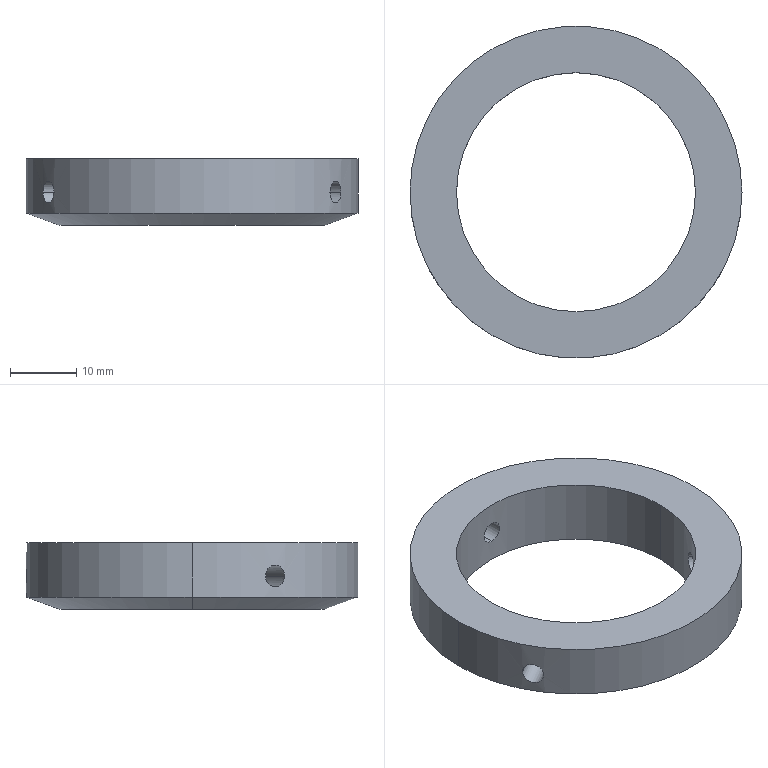Part | STEP file | 1 solid | 14 faces | box 50 x 50 x 10 mm | volume 8609 mm3 | cylinder 10 | cone 2 | plane 2 | commonest cylinder face diameters 3.3 x6 36 x2 50 x2